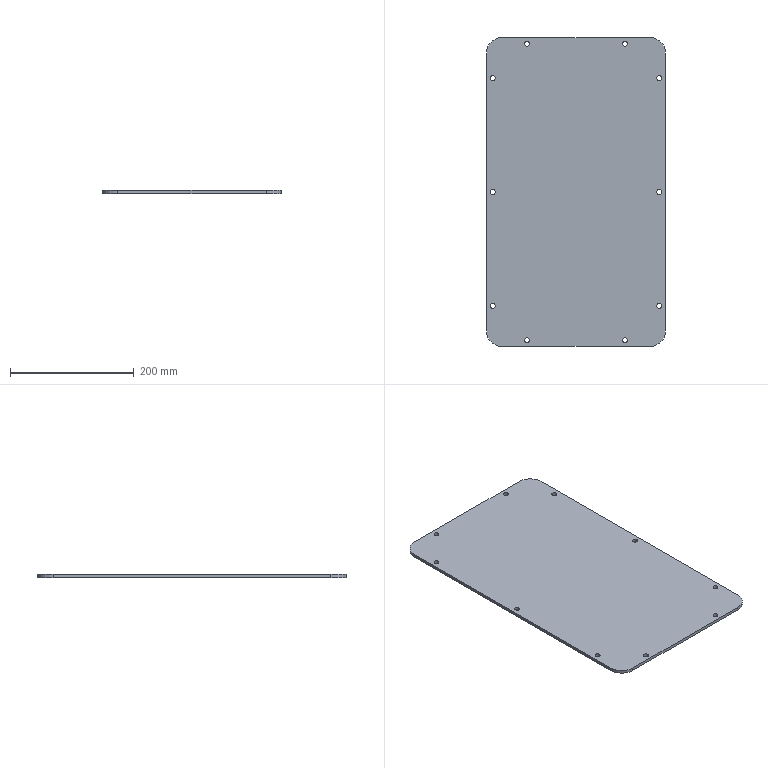Part | STEP file | PVC sealing plate | 1 solid | 30 faces | box 290 x 500 x 5 mm | volume 719804 mm3 | cylinder 24 | plane 6 | commonest cylinder face diameters 8 x20 50 x4